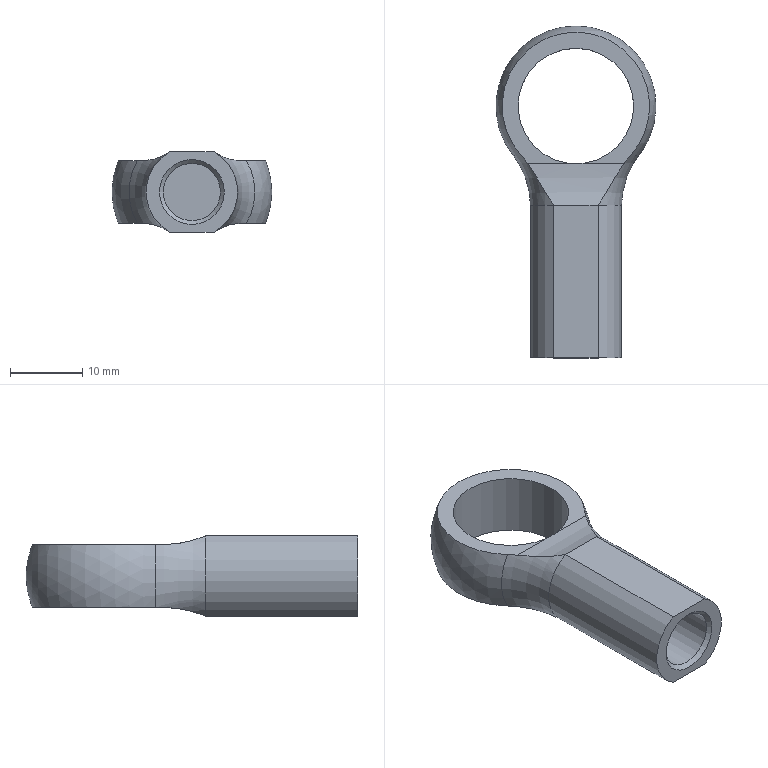Part | NX | features 4483T231 2 | 1 solid | 16 faces | box 22.225 x 46.038 x 11.113 mm | volume 3481 mm3 | plane 6 | cylinder 6 | torus 2 | cone 1 | sphere 1 | commonest cylinder face diameters 12.7 x2 29.369 x2 7.938 x1 16.034 x1
STEP:
#1=CARTESIAN_POINT('',(-6.679,7.919,-4.366));
#2=VERTEX_POINT('',#1);
#3=CARTESIAN_POINT('',(-7.561,9.001,-4.366));
#4=VERTEX_POINT('',#3);
#5=CARTESIAN_POINT('',(-6.679,7.919,-4.366));
#6=CARTESIAN_POINT('',(-6.954,8.297,-4.366));
#7=CARTESIAN_POINT('',(-7.249,8.657,-4.366));
#8=CARTESIAN_POINT('',(-7.561,9.001,-4.366));
#9=B_SPLINE_CURVE_WITH_KNOTS('',3,(#5,#6,#7,#8),.UNSPECIFIED.,.F.,.F.,(4,4),(0.004138,0.005535),.UNSPECIFIED.);
#10=EDGE_CURVE('',#2,#4,#9,.T.);
#11=ORIENTED_EDGE('',*,*,#10,.F.);
#12=CARTESIAN_POINT('',(-3.074,2.127,-5.556));
#13=VERTEX_POINT('',#12);
#14=CARTESIAN_POINT('',(-6.679,7.919,-4.366));
#15=CARTESIAN_POINT('',(-5.989,6.974,-4.366));
#16=CARTESIAN_POINT('',(-4.823,4.987,-4.549));
#17=CARTESIAN_POINT('',(-3.752,3.,-5.181));
#18=CARTESIAN_POINT('',(-3.074,2.127,-5.556));
#19=B_SPLINE_CURVE_WITH_KNOTS('',3,(#14,#15,#16,#17,#18),.UNSPECIFIED.,.F.,.F.,(4,1,4),(0.,0.003466,0.006932),.UNSPECIFIED.);
#20=EDGE_CURVE('',#2,#13,#19,.T.);
#21=ORIENTED_EDGE('',*,*,#20,.T.);
#22=CARTESIAN_POINT('',(-3.074,2.127,5.556));
#23=VERTEX_POINT('',#22);
#24=CARTESIAN_POINT('',(0.,2.127,0.));
#25=DIRECTION('',(0.,1.,0.));
#26=DIRECTION('',(-1.,0.,0.));
#27=AXIS2_PLACEMENT_3D('',#24,#25,#26);
#28=CIRCLE('',#27,6.35);
#29=EDGE_CURVE('',#13,#23,#28,.T.);
#30=ORIENTED_EDGE('',*,*,#29,.T.);
#31=CARTESIAN_POINT('',(-6.679,7.919,4.366));
#32=VERTEX_POINT('',#31);
#33=CARTESIAN_POINT('',(-3.074,2.127,5.556));
#34=CARTESIAN_POINT('',(-3.753,3.002,5.18));
#35=CARTESIAN_POINT('',(-4.81,4.965,4.554));
#36=CARTESIAN_POINT('',(-5.991,6.977,4.366));
#37=CARTESIAN_POINT('',(-6.679,7.919,4.366));
#38=B_SPLINE_CURVE_WITH_KNOTS('',3,(#33,#34,#35,#36,#37),.UNSPECIFIED.,.F.,.F.,(4,1,4),(0.,0.003467,0.006933),.UNSPECIFIED.);
#39=EDGE_CURVE('',#23,#32,#38,.T.);
#40=ORIENTED_EDGE('',*,*,#39,.T.);
#41=CARTESIAN_POINT('',(-7.561,9.001,4.366));
#42=VERTEX_POINT('',#41);
#43=CARTESIAN_POINT('',(-7.561,9.001,4.366));
#44=CARTESIAN_POINT('',(-7.248,8.656,4.366));
#45=CARTESIAN_POINT('',(-6.954,8.296,4.366));
#46=CARTESIAN_POINT('',(-6.679,7.919,4.366));
#47=B_SPLINE_CURVE_WITH_KNOTS('',3,(#43,#44,#45,#46),.UNSPECIFIED.,.F.,.F.,(4,4),(0.06597,0.06737),.UNSPECIFIED.);
#48=EDGE_CURVE('',#42,#32,#47,.T.);
#49=ORIENTED_EDGE('',*,*,#48,.F.);
#50=CARTESIAN_POINT('',(0.,9.001,0.));
#51=DIRECTION('',(0.,-1.,0.));
#52=DIRECTION('',(1.,0.,0.));
#53=AXIS2_PLACEMENT_3D('',#50,#51,#52);
#54=CIRCLE('',#53,8.731);
#55=EDGE_CURVE('',#42,#4,#54,.T.);
#56=ORIENTED_EDGE('',*,*,#55,.T.);
#57=EDGE_LOOP('',(#11,#21,#30,#40,#49,#56));
#58=FACE_BOUND('',#57,.T.);
#59=CARTESIAN_POINT('',(0.,2.127,0.));
#60=DIRECTION('',(0.,-1.,0.));
#61=DIRECTION('',(1.,0.,0.));
#62=AXIS2_PLACEMENT_3D('',#59,#60,#61);
#63=TOROIDAL_SURFACE('',#62,17.462,11.113);
#64=ADVANCED_FACE('',(#58),#63,.F.);
#65=CARTESIAN_POINT('',(4.5,-19.05,0.));
#66=VERTEX_POINT('',#65);
#67=CARTESIAN_POINT('',(0.,-19.05,0.));
#68=DIRECTION('',(0.,-1.,0.));
#69=DIRECTION('',(1.,0.,0.));
#70=AXIS2_PLACEMENT_3D('',#67,#68,#69);
#71=CIRCLE('',#70,4.5);
#72=EDGE_CURVE('',#66,#66,#71,.T.);
#73=ORIENTED_EDGE('',*,*,#72,.F.);
#74=EDGE_LOOP('',(#73));
#75=FACE_BOUND('',#74,.T.);
#76=CARTESIAN_POINT('',(-3.074,-19.05,-5.556));
#77=VERTEX_POINT('',#76);
#78=CARTESIAN_POINT('',(3.074,-19.05,-5.556));
#79=VERTEX_POINT('',#78);
#80=CARTESIAN_POINT('',(-5.556,-19.05,-5.556));
#81=DIRECTION('',(1.,0.,0.));
#82=VECTOR('',#81,1000.);
#83=LINE('',#80,#82);
#84=EDGE_CURVE('',#77,#79,#83,.T.);
#85=ORIENTED_EDGE('',*,*,#84,.T.);
#86=CARTESIAN_POINT('',(3.074,-19.05,5.556));
#87=VERTEX_POINT('',#86);
#88=CARTESIAN_POINT('',(0.,-19.05,0.));
#89=DIRECTION('',(0.,1.,0.));
#90=DIRECTION('',(-1.,0.,0.));
#91=AXIS2_PLACEMENT_3D('',#88,#89,#90);
#92=CIRCLE('',#91,6.35);
#93=EDGE_CURVE('',#87,#79,#92,.T.);
#94=ORIENTED_EDGE('',*,*,#93,.F.);
#95=CARTESIAN_POINT('',(-3.074,-19.05,5.556));
#96=VERTEX_POINT('',#95);
#97=CARTESIAN_POINT('',(-5.556,-19.05,5.556));
#98=DIRECTION('',(-1.,0.,0.));
#99=VECTOR('',#98,1000.);
#100=LINE('',#97,#99);
#101=EDGE_CURVE('',#87,#96,#100,.T.);
#102=ORIENTED_EDGE('',*,*,#101,.T.);
#103=CARTESIAN_POINT('',(0.,-19.05,0.));
#104=DIRECTION('',(0.,1.,0.));
#105=DIRECTION('',(-1.,0.,0.));
#106=AXIS2_PLACEMENT_3D('',#103,#104,#105);
#107=CIRCLE('',#106,6.35);
#108=EDGE_CURVE('',#77,#96,#107,.T.);
#109=ORIENTED_EDGE('',*,*,#108,.F.);
#110=EDGE_LOOP('',(#85,#94,#102,#109));
#111=FACE_BOUND('',#110,.T.);
#112=CARTESIAN_POINT('',(6.35,-19.05,0.));
#113=DIRECTION('',(0.,1.,0.));
#114=DIRECTION('',(-1.,0.,0.));
#115=AXIS2_PLACEMENT_3D('',#112,#113,#114);
#116=PLANE('',#115);
#117=ADVANCED_FACE('',(#75,#111),#116,.F.);
#118=CARTESIAN_POINT('',(-3.074,26.988,-5.556));
#119=DIRECTION('',(0.,1.,0.));
#120=VECTOR('',#119,1000.);
#121=LINE('',#118,#120);
#122=EDGE_CURVE('',#77,#13,#121,.T.);
#123=ORIENTED_EDGE('',*,*,#122,.F.);
#124=ORIENTED_EDGE('',*,*,#108,.T.);
#125=CARTESIAN_POINT('',(-3.074,26.988,5.556));
#126=DIRECTION('',(0.,1.,0.));
#127=VECTOR('',#126,1000.);
#128=LINE('',#125,#127);
#129=EDGE_CURVE('',#23,#96,#128,.F.);
#130=ORIENTED_EDGE('',*,*,#129,.F.);
#131=ORIENTED_EDGE('',*,*,#29,.F.);
#132=EDGE_LOOP('',(#123,#124,#130,#131));
#133=FACE_BOUND('',#132,.T.);
#134=CARTESIAN_POINT('',(0.,26.988,0.));
#135=DIRECTION('',(0.,1.,0.));
#136=DIRECTION('',(-1.,0.,0.));
#137=AXIS2_PLACEMENT_3D('',#134,#135,#136);
#138=CYLINDRICAL_SURFACE('',#137,6.35);
#139=ADVANCED_FACE('',(#133),#138,.T.);
#140=CARTESIAN_POINT('',(3.074,2.127,-5.556));
#141=VERTEX_POINT('',#140);
#142=CARTESIAN_POINT('',(3.074,26.988,-5.556));
#143=DIRECTION('',(0.,1.,0.));
#144=VECTOR('',#143,1000.);
#145=LINE('',#142,#144);
#146=EDGE_CURVE('',#141,#79,#145,.F.);
#147=ORIENTED_EDGE('',*,*,#146,.F.);
#148=CARTESIAN_POINT('',(3.074,2.127,5.556));
#149=VERTEX_POINT('',#148);
#150=CARTESIAN_POINT('',(0.,2.127,0.));
#151=DIRECTION('',(0.,1.,0.));
#152=DIRECTION('',(-1.,0.,0.));
#153=AXIS2_PLACEMENT_3D('',#150,#151,#152);
#154=CIRCLE('',#153,6.35);
#155=EDGE_CURVE('',#149,#141,#154,.T.);
#156=ORIENTED_EDGE('',*,*,#155,.F.);
#157=CARTESIAN_POINT('',(3.074,26.988,5.556));
#158=DIRECTION('',(0.,1.,0.));
#159=VECTOR('',#158,1000.);
#160=LINE('',#157,#159);
#161=EDGE_CURVE('',#87,#149,#160,.T.);
#162=ORIENTED_EDGE('',*,*,#161,.F.);
#163=ORIENTED_EDGE('',*,*,#93,.T.);
#164=EDGE_LOOP('',(#147,#156,#162,#163));
#165=FACE_BOUND('',#164,.T.);
#166=CARTESIAN_POINT('',(0.,26.988,0.));
#167=DIRECTION('',(0.,1.,0.));
#168=DIRECTION('',(-1.,0.,0.));
#169=AXIS2_PLACEMENT_3D('',#166,#167,#168);
#170=CYLINDRICAL_SURFACE('',#169,6.35);
#171=ADVANCED_FACE('',(#165),#170,.T.);
#172=ORIENTED_EDGE('',*,*,#161,.T.);
#173=CARTESIAN_POINT('',(0.,2.127,5.556));
#174=DIRECTION('',(-1.,0.,0.));
#175=VECTOR('',#174,1000.);
#176=LINE('',#173,#175);
#177=EDGE_CURVE('',#149,#23,#176,.T.);
#178=ORIENTED_EDGE('',*,*,#177,.T.);
#179=ORIENTED_EDGE('',*,*,#129,.T.);
#180=ORIENTED_EDGE('',*,*,#101,.F.);
#181=EDGE_LOOP('',(#172,#178,#179,#180));
#182=FACE_BOUND('',#181,.T.);
#183=CARTESIAN_POINT('',(-5.556,2.127,5.556));
#184=DIRECTION('',(0.,0.,1.));
#185=DIRECTION('',(1.,0.,0.));
#186=AXIS2_PLACEMENT_3D('',#183,#184,#185);
#187=PLANE('',#186);
#188=ADVANCED_FACE('',(#182),#187,.T.);
#189=ORIENTED_EDGE('',*,*,#122,.T.);
#190=CARTESIAN_POINT('',(0.,2.127,-5.556));
#191=DIRECTION('',(1.,0.,0.));
#192=VECTOR('',#191,1000.);
#193=LINE('',#190,#192);
#194=EDGE_CURVE('',#13,#141,#193,.T.);
#195=ORIENTED_EDGE('',*,*,#194,.T.);
#196=ORIENTED_EDGE('',*,*,#146,.T.);
#197=ORIENTED_EDGE('',*,*,#84,.F.);
#198=EDGE_LOOP('',(#189,#195,#196,#197));
#199=FACE_BOUND('',#198,.T.);
#200=CARTESIAN_POINT('',(-5.556,2.127,-5.556));
#201=DIRECTION('',(0.,0.,-1.));
#202=DIRECTION('',(-1.,0.,0.));
#203=AXIS2_PLACEMENT_3D('',#200,#201,#202);
#204=PLANE('',#203);
#205=ADVANCED_FACE('',(#199),#204,.T.);
#206=CARTESIAN_POINT('',(3.969,-18.518,0.));
#207=VERTEX_POINT('',#206);
#208=CARTESIAN_POINT('',(0.,-18.518,0.));
#209=DIRECTION('',(0.,-1.,0.));
#210=DIRECTION('',(1.,0.,0.));
#211=AXIS2_PLACEMENT_3D('',#208,#209,#210);
#212=CIRCLE('',#211,3.969);
#213=EDGE_CURVE('',#207,#207,#212,.F.);
#214=ORIENTED_EDGE('',*,*,#213,.T.);
#215=EDGE_LOOP('',(#214));
#216=FACE_BOUND('',#215,.T.);
#217=ORIENTED_EDGE('',*,*,#72,.T.);
#218=EDGE_LOOP('',(#217));
#219=FACE_BOUND('',#218,.T.);
#220=CARTESIAN_POINT('',(0.,-19.05,0.));
#221=DIRECTION('',(0.,-1.,0.));
#222=DIRECTION('',(1.,0.,0.));
#223=AXIS2_PLACEMENT_3D('',#220,#221,#222);
#224=CONICAL_SURFACE('',#223,4.5,0.7854);
#225=ADVANCED_FACE('',(#216,#219),#224,.F.);
#226=CARTESIAN_POINT('',(3.969,0.,0.));
#227=VERTEX_POINT('',#226);
#228=CARTESIAN_POINT('',(0.,0.,0.));
#229=DIRECTION('',(0.,-1.,0.));
#230=DIRECTION('',(1.,0.,0.));
#231=AXIS2_PLACEMENT_3D('',#228,#229,#230);
#232=CIRCLE('',#231,3.969);
#233=EDGE_CURVE('',#227,#227,#232,.T.);
#234=ORIENTED_EDGE('',*,*,#233,.F.);
#235=EDGE_LOOP('',(#234));
#236=FACE_BOUND('',#235,.T.);
#237=ORIENTED_EDGE('',*,*,#213,.F.);
#238=EDGE_LOOP('',(#237));
#239=FACE_BOUND('',#238,.T.);
#240=CARTESIAN_POINT('',(0.,0.,0.));
#241=DIRECTION('',(0.,-1.,0.));
#242=DIRECTION('',(1.,0.,0.));
#243=AXIS2_PLACEMENT_3D('',#240,#241,#242);
#244=CYLINDRICAL_SURFACE('',#243,3.969);
#245=ADVANCED_FACE('',(#236,#239),#244,.F.);
#246=ORIENTED_EDGE('',*,*,#233,.T.);
#247=EDGE_LOOP('',(#246));
#248=FACE_BOUND('',#247,.T.);
#249=CARTESIAN_POINT('',(3.969,0.,0.));
#250=DIRECTION('',(0.,1.,0.));
#251=DIRECTION('',(-1.,0.,0.));
#252=AXIS2_PLACEMENT_3D('',#249,#250,#251);
#253=PLANE('',#252);
#254=ADVANCED_FACE('',(#248),#253,.F.);
#255=CARTESIAN_POINT('',(7.561,9.001,-4.366));
#256=VERTEX_POINT('',#255);
#257=CARTESIAN_POINT('',(6.679,7.919,-4.366));
#258=VERTEX_POINT('',#257);
#259=CARTESIAN_POINT('',(7.561,9.001,-4.366));
#260=CARTESIAN_POINT('',(7.25,8.658,-4.366));
#261=CARTESIAN_POINT('',(6.953,8.295,-4.366));
#262=CARTESIAN_POINT('',(6.679,7.919,-4.366));
#263=B_SPLINE_CURVE_WITH_KNOTS('',3,(#259,#260,#261,#262),.UNSPECIFIED.,.F.,.F.,(4,4),(0.0648,0.06618),.UNSPECIFIED.);
#264=EDGE_CURVE('',#256,#258,#263,.T.);
#265=ORIENTED_EDGE('',*,*,#264,.F.);
#266=CARTESIAN_POINT('',(7.561,9.001,4.366));
#267=VERTEX_POINT('',#266);
#268=CARTESIAN_POINT('',(0.,9.001,0.));
#269=DIRECTION('',(0.,-1.,0.));
#270=DIRECTION('',(1.,0.,0.));
#271=AXIS2_PLACEMENT_3D('',#268,#269,#270);
#272=CIRCLE('',#271,8.731);
#273=EDGE_CURVE('',#256,#267,#272,.T.);
#274=ORIENTED_EDGE('',*,*,#273,.T.);
#275=CARTESIAN_POINT('',(6.679,7.919,4.366));
#276=VERTEX_POINT('',#275);
#277=CARTESIAN_POINT('',(6.679,7.919,4.366));
#278=CARTESIAN_POINT('',(6.952,8.294,4.366));
#279=CARTESIAN_POINT('',(7.247,8.655,4.366));
#280=CARTESIAN_POINT('',(7.561,9.001,4.366));
#281=B_SPLINE_CURVE_WITH_KNOTS('',3,(#277,#278,#279,#280),.UNSPECIFIED.,.F.,.F.,(4,4),(0.005227,0.006625),.UNSPECIFIED.);
#282=EDGE_CURVE('',#276,#267,#281,.T.);
#283=ORIENTED_EDGE('',*,*,#282,.F.);
#284=CARTESIAN_POINT('',(6.679,7.919,4.366));
#285=CARTESIAN_POINT('',(5.989,6.974,4.366));
#286=CARTESIAN_POINT('',(4.823,4.987,4.549));
#287=CARTESIAN_POINT('',(3.752,3.,5.181));
#288=CARTESIAN_POINT('',(3.074,2.127,5.556));
#289=B_SPLINE_CURVE_WITH_KNOTS('',3,(#284,#285,#286,#287,#288),.UNSPECIFIED.,.F.,.F.,(4,1,4),(0.,0.003466,0.006932),.UNSPECIFIED.);
#290=EDGE_CURVE('',#276,#149,#289,.T.);
#291=ORIENTED_EDGE('',*,*,#290,.T.);
#292=ORIENTED_EDGE('',*,*,#155,.T.);
#293=CARTESIAN_POINT('',(3.074,2.127,-5.556));
#294=CARTESIAN_POINT('',(3.753,3.002,-5.18));
#295=CARTESIAN_POINT('',(4.81,4.965,-4.554));
#296=CARTESIAN_POINT('',(5.991,6.977,-4.366));
#297=CARTESIAN_POINT('',(6.679,7.919,-4.366));
#298=B_SPLINE_CURVE_WITH_KNOTS('',3,(#293,#294,#295,#296,#297),.UNSPECIFIED.,.F.,.F.,(4,1,4),(0.,0.003467,0.006933),.UNSPECIFIED.);
#299=EDGE_CURVE('',#141,#258,#298,.T.);
#300=ORIENTED_EDGE('',*,*,#299,.T.);
#301=EDGE_LOOP('',(#265,#274,#283,#291,#292,#300));
#302=FACE_BOUND('',#301,.T.);
#303=CARTESIAN_POINT('',(0.,2.127,0.));
#304=DIRECTION('',(0.,-1.,0.));
#305=DIRECTION('',(1.,0.,0.));
#306=AXIS2_PLACEMENT_3D('',#303,#304,#305);
#307=TOROIDAL_SURFACE('',#306,17.462,11.113);
#308=ADVANCED_FACE('',(#302),#307,.F.);
#309=CARTESIAN_POINT('',(0.,15.875,-4.366));
#310=DIRECTION('',(0.,0.,1.));
#311=DIRECTION('',(0.,-1.,0.));
#312=AXIS2_PLACEMENT_3D('',#309,#310,#311);
#313=CIRCLE('',#312,10.219);
#314=EDGE_CURVE('',#4,#256,#313,.F.);
#315=ORIENTED_EDGE('',*,*,#314,.F.);
#316=ORIENTED_EDGE('',*,*,#55,.F.);
#317=CARTESIAN_POINT('',(0.,15.875,4.366));
#318=DIRECTION('',(0.,0.,-1.));
#319=DIRECTION('',(0.,1.,0.));
#320=AXIS2_PLACEMENT_3D('',#317,#318,#319);
#321=CIRCLE('',#320,10.219);
#322=EDGE_CURVE('',#267,#42,#321,.F.);
#323=ORIENTED_EDGE('',*,*,#322,.F.);
#324=ORIENTED_EDGE('',*,*,#273,.F.);
#325=EDGE_LOOP('',(#315,#316,#323,#324));
#326=FACE_BOUND('',#325,.T.);
#327=CARTESIAN_POINT('',(0.,15.875,0.));
#328=DIRECTION('',(0.,-1.,0.));
#329=DIRECTION('',(1.,0.,0.));
#330=AXIS2_PLACEMENT_3D('',#327,#328,#329);
#331=SPHERICAL_SURFACE('',#330,11.113);
#332=ADVANCED_FACE('',(#326),#331,.T.);
#333=CARTESIAN_POINT('',(-0.9865,7.919,4.366));
#334=VERTEX_POINT('',#333);
#335=CARTESIAN_POINT('',(-11.113,7.919,4.366));
#336=DIRECTION('',(-1.,0.,0.));
#337=VECTOR('',#336,1000.);
#338=LINE('',#335,#337);
#339=EDGE_CURVE('',#32,#334,#338,.F.);
#340=ORIENTED_EDGE('',*,*,#339,.T.);
#341=CARTESIAN_POINT('',(0.9865,7.919,4.366));
#342=VERTEX_POINT('',#341);
#343=CARTESIAN_POINT('',(0.,15.875,4.366));
#344=DIRECTION('',(0.,0.,-1.));
#345=DIRECTION('',(0.,1.,0.));
#346=AXIS2_PLACEMENT_3D('',#343,#344,#345);
#347=CIRCLE('',#346,8.017);
#348=EDGE_CURVE('',#334,#342,#347,.T.);
#349=ORIENTED_EDGE('',*,*,#348,.T.);
#350=CARTESIAN_POINT('',(-11.113,7.919,4.366));
#351=DIRECTION('',(-1.,0.,0.));
#352=VECTOR('',#351,1000.);
#353=LINE('',#350,#352);
#354=EDGE_CURVE('',#342,#276,#353,.F.);
#355=ORIENTED_EDGE('',*,*,#354,.T.);
#356=ORIENTED_EDGE('',*,*,#282,.T.);
#357=ORIENTED_EDGE('',*,*,#322,.T.);
#358=ORIENTED_EDGE('',*,*,#48,.T.);
#359=EDGE_LOOP('',(#340,#349,#355,#356,#357,#358));
#360=FACE_BOUND('',#359,.T.);
#361=CARTESIAN_POINT('',(-11.113,26.988,4.366));
#362=DIRECTION('',(0.,0.,-1.));
#363=DIRECTION('',(0.,1.,0.));
#364=AXIS2_PLACEMENT_3D('',#361,#362,#363);
#365=PLANE('',#364);
#366=ADVANCED_FACE('',(#360),#365,.F.);
#367=CARTESIAN_POINT('',(0.9865,7.919,-4.366));
#368=VERTEX_POINT('',#367);
#369=CARTESIAN_POINT('',(-11.113,7.919,-4.366));
#370=DIRECTION('',(1.,0.,0.));
#371=VECTOR('',#370,1000.);
#372=LINE('',#369,#371);
#373=EDGE_CURVE('',#258,#368,#372,.F.);
#374=ORIENTED_EDGE('',*,*,#373,.T.);
#375=CARTESIAN_POINT('',(-0.9865,7.919,-4.366));
#376=VERTEX_POINT('',#375);
#377=CARTESIAN_POINT('',(0.,15.875,-4.366));
#378=DIRECTION('',(0.,0.,1.));
#379=DIRECTION('',(0.,-1.,0.));
#380=AXIS2_PLACEMENT_3D('',#377,#378,#379);
#381=CIRCLE('',#380,8.017);
#382=EDGE_CURVE('',#368,#376,#381,.T.);
#383=ORIENTED_EDGE('',*,*,#382,.T.);
#384=CARTESIAN_POINT('',(-11.113,7.919,-4.366));
#385=DIRECTION('',(1.,0.,0.));
#386=VECTOR('',#385,1000.);
#387=LINE('',#384,#386);
#388=EDGE_CURVE('',#376,#2,#387,.F.);
#389=ORIENTED_EDGE('',*,*,#388,.T.);
#390=ORIENTED_EDGE('',*,*,#10,.T.);
#391=ORIENTED_EDGE('',*,*,#314,.T.);
#392=ORIENTED_EDGE('',*,*,#264,.T.);
#393=EDGE_LOOP('',(#374,#383,#389,#390,#391,#392));
#394=FACE_BOUND('',#393,.T.);
#395=CARTESIAN_POINT('',(-11.113,26.988,-4.366));
#396=DIRECTION('',(0.,0.,1.));
#397=DIRECTION('',(0.,-1.,0.));
#398=AXIS2_PLACEMENT_3D('',#395,#396,#397);
#399=PLANE('',#398);
#400=ADVANCED_FACE('',(#394),#399,.F.);
#401=ORIENTED_EDGE('',*,*,#354,.F.);
#402=CARTESIAN_POINT('',(0.9865,7.919,4.366));
#403=CARTESIAN_POINT('',(0.3288,7.838,4.366));
#404=CARTESIAN_POINT('',(-0.3288,7.838,4.366));
#405=CARTESIAN_POINT('',(-0.9865,7.919,4.366));
#406=B_SPLINE_CURVE_WITH_KNOTS('',3,(#402,#403,#404,#405),.UNSPECIFIED.,.F.,.F.,(4,4),(0.,0.001973),.UNSPECIFIED.);
#407=EDGE_CURVE('',#342,#334,#406,.T.);
#408=ORIENTED_EDGE('',*,*,#407,.T.);
#409=ORIENTED_EDGE('',*,*,#339,.F.);
#410=ORIENTED_EDGE('',*,*,#39,.F.);
#411=ORIENTED_EDGE('',*,*,#177,.F.);
#412=ORIENTED_EDGE('',*,*,#290,.F.);
#413=EDGE_LOOP('',(#401,#408,#409,#410,#411,#412));
#414=FACE_BOUND('',#413,.T.);
#415=CARTESIAN_POINT('',(-11.113,7.919,19.05));
#416=DIRECTION('',(-1.,0.,0.));
#417=DIRECTION('',(0.,0.,1.));
#418=AXIS2_PLACEMENT_3D('',#415,#416,#417);
#419=CYLINDRICAL_SURFACE('',#418,14.684);
#420=ADVANCED_FACE('',(#414),#419,.F.);
#421=ORIENTED_EDGE('',*,*,#388,.F.);
#422=CARTESIAN_POINT('',(-0.9865,7.919,-4.366));
#423=CARTESIAN_POINT('',(-0.3288,7.838,-4.366));
#424=CARTESIAN_POINT('',(0.3288,7.838,-4.366));
#425=CARTESIAN_POINT('',(0.9865,7.919,-4.366));
#426=B_SPLINE_CURVE_WITH_KNOTS('',3,(#422,#423,#424,#425),.UNSPECIFIED.,.F.,.F.,(4,4),(0.,0.001973),.UNSPECIFIED.);
#427=EDGE_CURVE('',#376,#368,#426,.T.);
#428=ORIENTED_EDGE('',*,*,#427,.T.);
#429=ORIENTED_EDGE('',*,*,#373,.F.);
#430=ORIENTED_EDGE('',*,*,#299,.F.);
#431=ORIENTED_EDGE('',*,*,#194,.F.);
#432=ORIENTED_EDGE('',*,*,#20,.F.);
#433=EDGE_LOOP('',(#421,#428,#429,#430,#431,#432));
#434=FACE_BOUND('',#433,.T.);
#435=CARTESIAN_POINT('',(-11.113,7.919,-19.05));
#436=DIRECTION('',(1.,0.,0.));
#437=DIRECTION('',(0.,0.,-1.));
#438=AXIS2_PLACEMENT_3D('',#435,#436,#437);
#439=CYLINDRICAL_SURFACE('',#438,14.684);
#440=ADVANCED_FACE('',(#434),#439,.F.);
#441=ORIENTED_EDGE('',*,*,#427,.F.);
#442=ORIENTED_EDGE('',*,*,#382,.F.);
#443=EDGE_LOOP('',(#441,#442));
#444=FACE_BOUND('',#443,.T.);
#445=ORIENTED_EDGE('',*,*,#407,.F.);
#446=ORIENTED_EDGE('',*,*,#348,.F.);
#447=EDGE_LOOP('',(#445,#446));
#448=FACE_BOUND('',#447,.T.);
#449=CARTESIAN_POINT('',(0.,15.875,-6.389));
#450=DIRECTION('',(0.,0.,1.));
#451=DIRECTION('',(1.,0.,0.));
#452=AXIS2_PLACEMENT_3D('',#449,#450,#451);
#453=CYLINDRICAL_SURFACE('',#452,8.017);
#454=ADVANCED_FACE('',(#444,#448),#453,.F.);
#455=CLOSED_SHELL('',(#64,#117,#139,#171,#188,#205,#225,#245,#254,#308,#332,#366,#400,#420,#440,#454));
#456=MANIFOLD_SOLID_BREP('',#455);
#457=(LENGTH_UNIT()NAMED_UNIT(*)SI_UNIT(.MILLI.,.METRE.));
#458=UNCERTAINTY_MEASURE_WITH_UNIT(LENGTH_MEASURE(0.0508),#457,'','');
#459=(NAMED_UNIT(*)PLANE_ANGLE_UNIT()SI_UNIT($,.RADIAN.));
#460=(NAMED_UNIT(*)SI_UNIT($,.STERADIAN.)SOLID_ANGLE_UNIT());
#461=(GEOMETRIC_REPRESENTATION_CONTEXT(3)GLOBAL_UNCERTAINTY_ASSIGNED_CONTEXT((#458))GLOBAL_UNIT_ASSIGNED_CONTEXT((#457,#459,#460))REPRESENTATION_CONTEXT('',''));
#462=ADVANCED_BREP_SHAPE_REPRESENTATION('',(#456),#461);